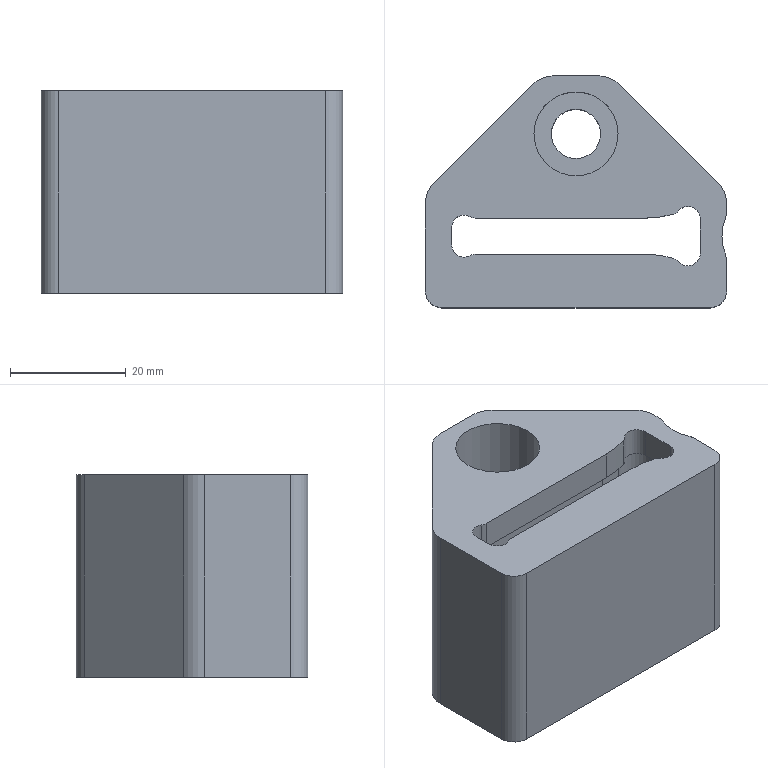Part | NX | features DIE-81 2 | 1 solid | 50 faces | box 52 x 40 x 35 mm | volume 42492 mm3 | cylinder 25 | plane 19 | spline 6 | commonest cylinder face diameters 1.76 x4 3.76 x4 4.24 x4 6.24 x4 10 x4 6 x2